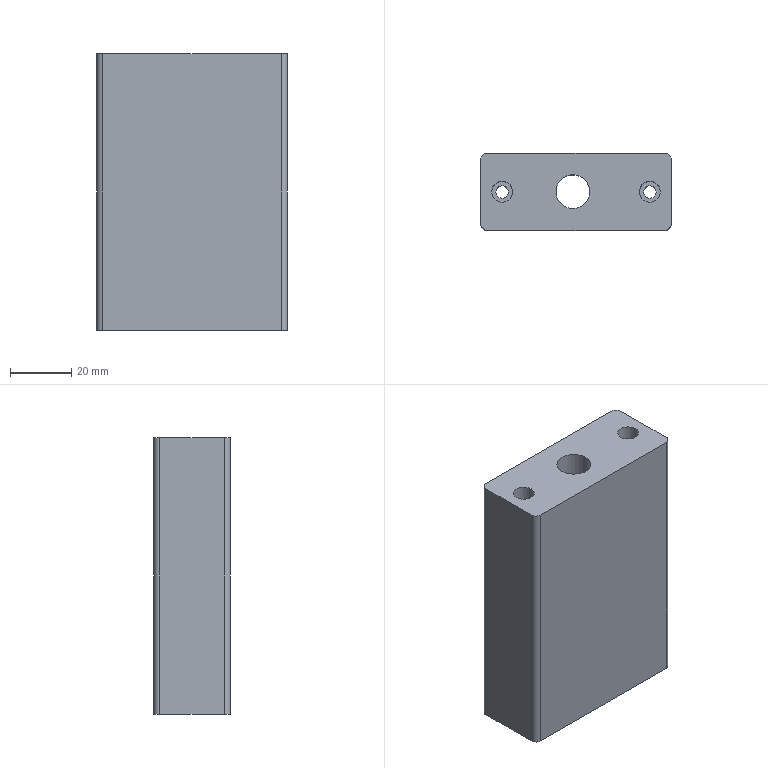Part | STEP file | gslz 2016.10.28-10_id2890_x_t | 1 solid | 19 faces | box 62 x 25 x 90 mm | volume 116529 mm3 | cylinder 10 | plane 9 | commonest cylinder face diameters 4 x4 4.1 x2 6.8 x2 11 x1 17 x1
STEP:
#1=CARTESIAN_POINT('',(0.,0.,0.));
#2=DIRECTION('',(0.,0.,1.));
#3=DIRECTION('',(1.,0.,0.));
#4=AXIS2_PLACEMENT_3D('',#1,#2,#3);
#5=CARTESIAN_POINT('',(1002.,-173.5,85.));
#6=VERTEX_POINT('',#5);
#7=CARTESIAN_POINT('',(1060.,-173.5,85.));
#8=VERTEX_POINT('',#7);
#9=CARTESIAN_POINT('',(1140.635,-173.5,85.));
#10=DIRECTION('',(1.,0.,0.));
#11=VECTOR('',#10,1.);
#12=LINE('',#9,#11);
#13=CARTESIAN_POINT('',(1030.,-162.5,85.));
#14=DIRECTION('',(0.,0.,1.));
#15=DIRECTION('',(-1.,0.,0.));
#16=AXIS2_PLACEMENT_3D('',#13,#14,#15);
#17=PLANE('',#16);
#18=CARTESIAN_POINT('',(-110.635,11.));
#19=DIRECTION('',(-1.,0.));
#20=VECTOR('',#19,1.);
#21=LINE('',#18,#20);
#22=(GEOMETRIC_REPRESENTATION_CONTEXT(2)PARAMETRIC_REPRESENTATION_CONTEXT()REPRESENTATION_CONTEXT('',''));
#23=DEFINITIONAL_REPRESENTATION('',(#21),#22);
#24=PCURVE('',#17,#23);
#25=CARTESIAN_POINT('',(1140.635,-173.5,80.));
#26=DIRECTION('',(0.,1.,0.));
#27=DIRECTION('',(0.,0.,-1.));
#28=AXIS2_PLACEMENT_3D('',#25,#26,#27);
#29=PLANE('',#28);
#30=CARTESIAN_POINT('',(-5.,0.));
#31=DIRECTION('',(0.,-1.));
#32=VECTOR('',#31,1.);
#33=LINE('',#30,#32);
#34=(GEOMETRIC_REPRESENTATION_CONTEXT(2)PARAMETRIC_REPRESENTATION_CONTEXT()REPRESENTATION_CONTEXT('',''));
#35=DEFINITIONAL_REPRESENTATION('',(#33),#34);
#36=PCURVE('',#29,#35);
#37=SURFACE_CURVE('',#12,(#24,#36),.PCURVE_S1.);
#38=EDGE_CURVE('',#6,#8,#37,.T.);
#39=ORIENTED_EDGE('',*,*,#38,.T.);
#40=CARTESIAN_POINT('',(1062.,-171.5,85.));
#41=VERTEX_POINT('',#40);
#42=CARTESIAN_POINT('',(1060.,-171.5,85.));
#43=DIRECTION('',(0.,0.,1.));
#44=DIRECTION('',(1.,0.,0.));
#45=AXIS2_PLACEMENT_3D('',#42,#43,#44);
#46=CIRCLE('',#45,2.);
#47=CARTESIAN_POINT('',(-30.,9.));
#48=DIRECTION('',(-1.,0.));
#49=AXIS2_PLACEMENT_2D('',#47,#48);
#50=CIRCLE('',#49,2.);
#51=(GEOMETRIC_REPRESENTATION_CONTEXT(2)PARAMETRIC_REPRESENTATION_CONTEXT()REPRESENTATION_CONTEXT('',''));
#52=DEFINITIONAL_REPRESENTATION('',(#50),#51);
#53=PCURVE('',#17,#52);
#54=CARTESIAN_POINT('',(1060.,-171.5,80.));
#55=DIRECTION('',(0.,0.,1.));
#56=DIRECTION('',(-1.,0.,0.));
#57=AXIS2_PLACEMENT_3D('',#54,#55,#56);
#58=CYLINDRICAL_SURFACE('',#57,2.);
#59=CARTESIAN_POINT('',(-3.142,5.));
#60=DIRECTION('',(1.,0.));
#61=VECTOR('',#60,1.);
#62=LINE('',#59,#61);
#63=(GEOMETRIC_REPRESENTATION_CONTEXT(2)PARAMETRIC_REPRESENTATION_CONTEXT()REPRESENTATION_CONTEXT('',''));
#64=DEFINITIONAL_REPRESENTATION('',(#62),#63);
#65=PCURVE('',#58,#64);
#66=SURFACE_CURVE('',#46,(#53,#65),.PCURVE_S1.);
#67=EDGE_CURVE('',#8,#41,#66,.T.);
#68=ORIENTED_EDGE('',*,*,#67,.T.);
#69=CARTESIAN_POINT('',(1062.,-150.5,85.));
#70=VERTEX_POINT('',#69);
#71=CARTESIAN_POINT('',(1062.,-161.,85.));
#72=DIRECTION('',(0.,1.,0.));
#73=VECTOR('',#72,1.);
#74=LINE('',#71,#73);
#75=CARTESIAN_POINT('',(-32.,-1.5));
#76=DIRECTION('',(0.,-1.));
#77=VECTOR('',#76,1.);
#78=LINE('',#75,#77);
#79=(GEOMETRIC_REPRESENTATION_CONTEXT(2)PARAMETRIC_REPRESENTATION_CONTEXT()REPRESENTATION_CONTEXT('',''));
#80=DEFINITIONAL_REPRESENTATION('',(#78),#79);
#81=PCURVE('',#17,#80);
#82=CARTESIAN_POINT('',(1062.,-161.,46.));
#83=DIRECTION('',(-1.,0.,0.));
#84=DIRECTION('',(0.,0.,-1.));
#85=AXIS2_PLACEMENT_3D('',#82,#83,#84);
#86=PLANE('',#85);
#87=CARTESIAN_POINT('',(-39.,0.));
#88=DIRECTION('',(0.,-1.));
#89=VECTOR('',#88,1.);
#90=LINE('',#87,#89);
#91=(GEOMETRIC_REPRESENTATION_CONTEXT(2)PARAMETRIC_REPRESENTATION_CONTEXT()REPRESENTATION_CONTEXT('',''));
#92=DEFINITIONAL_REPRESENTATION('',(#90),#91);
#93=PCURVE('',#86,#92);
#94=SURFACE_CURVE('',#74,(#81,#93),.PCURVE_S1.);
#95=EDGE_CURVE('',#41,#70,#94,.T.);
#96=ORIENTED_EDGE('',*,*,#95,.T.);
#97=CARTESIAN_POINT('',(1060.,-148.5,85.));
#98=VERTEX_POINT('',#97);
#99=CARTESIAN_POINT('',(1060.,-150.5,85.));
#100=DIRECTION('',(0.,0.,1.));
#101=DIRECTION('',(1.,0.,0.));
#102=AXIS2_PLACEMENT_3D('',#99,#100,#101);
#103=CIRCLE('',#102,2.);
#104=CARTESIAN_POINT('',(-30.,-12.));
#105=DIRECTION('',(-1.,0.));
#106=AXIS2_PLACEMENT_2D('',#104,#105);
#107=CIRCLE('',#106,2.);
#108=(GEOMETRIC_REPRESENTATION_CONTEXT(2)PARAMETRIC_REPRESENTATION_CONTEXT()REPRESENTATION_CONTEXT('',''));
#109=DEFINITIONAL_REPRESENTATION('',(#107),#108);
#110=PCURVE('',#17,#109);
#111=CARTESIAN_POINT('',(1060.,-150.5,46.));
#112=DIRECTION('',(0.,0.,1.));
#113=DIRECTION('',(-1.,0.,0.));
#114=AXIS2_PLACEMENT_3D('',#111,#112,#113);
#115=CYLINDRICAL_SURFACE('',#114,2.);
#116=CARTESIAN_POINT('',(3.142,39.));
#117=DIRECTION('',(1.,0.));
#118=VECTOR('',#117,1.);
#119=LINE('',#116,#118);
#120=(GEOMETRIC_REPRESENTATION_CONTEXT(2)PARAMETRIC_REPRESENTATION_CONTEXT()REPRESENTATION_CONTEXT('',''));
#121=DEFINITIONAL_REPRESENTATION('',(#119),#120);
#122=PCURVE('',#115,#121);
#123=SURFACE_CURVE('',#103,(#110,#122),.PCURVE_S1.);
#124=EDGE_CURVE('',#70,#98,#123,.T.);
#125=ORIENTED_EDGE('',*,*,#124,.T.);
#126=CARTESIAN_POINT('',(1002.,-148.5,85.));
#127=VERTEX_POINT('',#126);
#128=CARTESIAN_POINT('',(405.,-148.5,85.));
#129=DIRECTION('',(-1.,0.,0.));
#130=VECTOR('',#129,1.);
#131=LINE('',#128,#130);
#132=CARTESIAN_POINT('',(625.,-14.));
#133=DIRECTION('',(1.,0.));
#134=VECTOR('',#133,1.);
#135=LINE('',#132,#134);
#136=(GEOMETRIC_REPRESENTATION_CONTEXT(2)PARAMETRIC_REPRESENTATION_CONTEXT()REPRESENTATION_CONTEXT('',''));
#137=DEFINITIONAL_REPRESENTATION('',(#135),#136);
#138=PCURVE('',#17,#137);
#139=CARTESIAN_POINT('',(405.,-148.5,80.));
#140=DIRECTION('',(0.,-1.,0.));
#141=DIRECTION('',(0.,0.,1.));
#142=AXIS2_PLACEMENT_3D('',#139,#140,#141);
#143=PLANE('',#142);
#144=CARTESIAN_POINT('',(5.,0.));
#145=DIRECTION('',(0.,1.));
#146=VECTOR('',#145,1.);
#147=LINE('',#144,#146);
#148=(GEOMETRIC_REPRESENTATION_CONTEXT(2)PARAMETRIC_REPRESENTATION_CONTEXT()REPRESENTATION_CONTEXT('',''));
#149=DEFINITIONAL_REPRESENTATION('',(#147),#148);
#150=PCURVE('',#143,#149);
#151=SURFACE_CURVE('',#131,(#138,#150),.PCURVE_S1.);
#152=EDGE_CURVE('',#98,#127,#151,.T.);
#153=ORIENTED_EDGE('',*,*,#152,.T.);
#154=CARTESIAN_POINT('',(1000.,-150.5,85.));
#155=VERTEX_POINT('',#154);
#156=CARTESIAN_POINT('',(1002.,-150.5,85.));
#157=DIRECTION('',(0.,0.,1.));
#158=DIRECTION('',(1.,0.,0.));
#159=AXIS2_PLACEMENT_3D('',#156,#157,#158);
#160=CIRCLE('',#159,2.);
#161=CARTESIAN_POINT('',(28.,-12.));
#162=DIRECTION('',(-1.,0.));
#163=AXIS2_PLACEMENT_2D('',#161,#162);
#164=CIRCLE('',#163,2.);
#165=(GEOMETRIC_REPRESENTATION_CONTEXT(2)PARAMETRIC_REPRESENTATION_CONTEXT()REPRESENTATION_CONTEXT('',''));
#166=DEFINITIONAL_REPRESENTATION('',(#164),#165);
#167=PCURVE('',#17,#166);
#168=CARTESIAN_POINT('',(1002.,-150.5,80.));
#169=DIRECTION('',(0.,0.,1.));
#170=DIRECTION('',(-1.,0.,0.));
#171=AXIS2_PLACEMENT_3D('',#168,#169,#170);
#172=CYLINDRICAL_SURFACE('',#171,2.);
#173=CARTESIAN_POINT('',(3.142,5.));
#174=DIRECTION('',(1.,0.));
#175=VECTOR('',#174,1.);
#176=LINE('',#173,#175);
#177=(GEOMETRIC_REPRESENTATION_CONTEXT(2)PARAMETRIC_REPRESENTATION_CONTEXT()REPRESENTATION_CONTEXT('',''));
#178=DEFINITIONAL_REPRESENTATION('',(#176),#177);
#179=PCURVE('',#172,#178);
#180=SURFACE_CURVE('',#160,(#167,#179),.PCURVE_S1.);
#181=EDGE_CURVE('',#127,#155,#180,.T.);
#182=ORIENTED_EDGE('',*,*,#181,.T.);
#183=CARTESIAN_POINT('',(1000.,-171.5,85.));
#184=VERTEX_POINT('',#183);
#185=CARTESIAN_POINT('',(1000.,-154.5,85.));
#186=DIRECTION('',(0.,1.,0.));
#187=VECTOR('',#186,1.);
#188=LINE('',#185,#187);
#189=CARTESIAN_POINT('',(30.,-8.));
#190=DIRECTION('',(0.,-1.));
#191=VECTOR('',#190,1.);
#192=LINE('',#189,#191);
#193=(GEOMETRIC_REPRESENTATION_CONTEXT(2)PARAMETRIC_REPRESENTATION_CONTEXT()REPRESENTATION_CONTEXT('',''));
#194=DEFINITIONAL_REPRESENTATION('',(#192),#193);
#195=PCURVE('',#17,#194);
#196=CARTESIAN_POINT('',(1000.,-154.5,80.));
#197=DIRECTION('',(-1.,0.,0.));
#198=DIRECTION('',(0.,0.,-1.));
#199=AXIS2_PLACEMENT_3D('',#196,#197,#198);
#200=PLANE('',#199);
#201=CARTESIAN_POINT('',(-5.,0.));
#202=DIRECTION('',(0.,-1.));
#203=VECTOR('',#202,1.);
#204=LINE('',#201,#203);
#205=(GEOMETRIC_REPRESENTATION_CONTEXT(2)PARAMETRIC_REPRESENTATION_CONTEXT()REPRESENTATION_CONTEXT('',''));
#206=DEFINITIONAL_REPRESENTATION('',(#204),#205);
#207=PCURVE('',#200,#206);
#208=SURFACE_CURVE('',#188,(#195,#207),.PCURVE_S1.);
#209=EDGE_CURVE('',#184,#155,#208,.T.);
#210=ORIENTED_EDGE('',*,*,#209,.F.);
#211=CARTESIAN_POINT('',(1002.,-171.5,85.));
#212=DIRECTION('',(0.,0.,1.));
#213=DIRECTION('',(1.,0.,0.));
#214=AXIS2_PLACEMENT_3D('',#211,#212,#213);
#215=CIRCLE('',#214,2.);
#216=CARTESIAN_POINT('',(28.,9.));
#217=DIRECTION('',(-1.,0.));
#218=AXIS2_PLACEMENT_2D('',#216,#217);
#219=CIRCLE('',#218,2.);
#220=(GEOMETRIC_REPRESENTATION_CONTEXT(2)PARAMETRIC_REPRESENTATION_CONTEXT()REPRESENTATION_CONTEXT('',''));
#221=DEFINITIONAL_REPRESENTATION('',(#219),#220);
#222=PCURVE('',#17,#221);
#223=CARTESIAN_POINT('',(1002.,-171.5,80.));
#224=DIRECTION('',(0.,0.,1.));
#225=DIRECTION('',(-1.,0.,0.));
#226=AXIS2_PLACEMENT_3D('',#223,#224,#225);
#227=CYLINDRICAL_SURFACE('',#226,2.);
#228=CARTESIAN_POINT('',(-3.142,5.));
#229=DIRECTION('',(1.,0.));
#230=VECTOR('',#229,1.);
#231=LINE('',#228,#230);
#232=(GEOMETRIC_REPRESENTATION_CONTEXT(2)PARAMETRIC_REPRESENTATION_CONTEXT()REPRESENTATION_CONTEXT('',''));
#233=DEFINITIONAL_REPRESENTATION('',(#231),#232);
#234=PCURVE('',#227,#233);
#235=SURFACE_CURVE('',#215,(#222,#234),.PCURVE_S1.);
#236=EDGE_CURVE('',#184,#6,#235,.T.);
#237=ORIENTED_EDGE('',*,*,#236,.T.);
#238=EDGE_LOOP('',(#39,#68,#96,#125,#153,#182,#210,#237));
#239=FACE_BOUND('',#238,.T.);
#240=CARTESIAN_POINT('',(1035.5,-161.,85.));
#241=VERTEX_POINT('',#240);
#242=CARTESIAN_POINT('',(1030.,-161.,85.));
#243=DIRECTION('',(0.,0.,1.));
#244=DIRECTION('',(1.,0.,0.));
#245=AXIS2_PLACEMENT_3D('',#242,#243,#244);
#246=CIRCLE('',#245,5.5);
#247=CARTESIAN_POINT('',(0.,-1.5));
#248=DIRECTION('',(-1.,0.));
#249=AXIS2_PLACEMENT_2D('',#247,#248);
#250=CIRCLE('',#249,5.5);
#251=(GEOMETRIC_REPRESENTATION_CONTEXT(2)PARAMETRIC_REPRESENTATION_CONTEXT()REPRESENTATION_CONTEXT('',''));
#252=DEFINITIONAL_REPRESENTATION('',(#250),#251);
#253=PCURVE('',#17,#252);
#254=CARTESIAN_POINT('',(1030.,-161.,-13.));
#255=DIRECTION('',(0.,0.,1.));
#256=DIRECTION('',(1.,0.,0.));
#257=AXIS2_PLACEMENT_3D('',#254,#255,#256);
#258=CYLINDRICAL_SURFACE('',#257,5.5);
#259=CARTESIAN_POINT('',(0.,98.));
#260=DIRECTION('',(1.,0.));
#261=VECTOR('',#260,1.);
#262=LINE('',#259,#261);
#263=(GEOMETRIC_REPRESENTATION_CONTEXT(2)PARAMETRIC_REPRESENTATION_CONTEXT()REPRESENTATION_CONTEXT('',''));
#264=DEFINITIONAL_REPRESENTATION('',(#262),#263);
#265=PCURVE('',#258,#264);
#266=SURFACE_CURVE('',#246,(#253,#265),.PCURVE_S1.);
#267=EDGE_CURVE('',#241,#241,#266,.T.);
#268=ORIENTED_EDGE('',*,*,#267,.F.);
#269=EDGE_LOOP('',(#268));
#270=FACE_BOUND('',#269,.T.);
#271=CARTESIAN_POINT('',(1010.4,-161.,85.));
#272=VERTEX_POINT('',#271);
#273=CARTESIAN_POINT('',(1007.,-161.,85.));
#274=DIRECTION('',(0.,0.,1.));
#275=DIRECTION('',(1.,0.,0.));
#276=AXIS2_PLACEMENT_3D('',#273,#274,#275);
#277=CIRCLE('',#276,3.4);
#278=CARTESIAN_POINT('',(23.,-1.5));
#279=DIRECTION('',(-1.,0.));
#280=AXIS2_PLACEMENT_2D('',#278,#279);
#281=CIRCLE('',#280,3.4);
#282=(GEOMETRIC_REPRESENTATION_CONTEXT(2)PARAMETRIC_REPRESENTATION_CONTEXT()REPRESENTATION_CONTEXT('',''));
#283=DEFINITIONAL_REPRESENTATION('',(#281),#282);
#284=PCURVE('',#17,#283);
#285=CARTESIAN_POINT('',(1007.,-161.,36.));
#286=DIRECTION('',(0.,0.,1.));
#287=DIRECTION('',(1.,0.,0.));
#288=AXIS2_PLACEMENT_3D('',#285,#286,#287);
#289=CYLINDRICAL_SURFACE('',#288,3.4);
#290=CARTESIAN_POINT('',(0.,49.));
#291=DIRECTION('',(1.,0.));
#292=VECTOR('',#291,1.);
#293=LINE('',#290,#292);
#294=(GEOMETRIC_REPRESENTATION_CONTEXT(2)PARAMETRIC_REPRESENTATION_CONTEXT()REPRESENTATION_CONTEXT('',''));
#295=DEFINITIONAL_REPRESENTATION('',(#293),#294);
#296=PCURVE('',#289,#295);
#297=SURFACE_CURVE('',#277,(#284,#296),.PCURVE_S1.);
#298=EDGE_CURVE('',#272,#272,#297,.T.);
#299=ORIENTED_EDGE('',*,*,#298,.F.);
#300=EDGE_LOOP('',(#299));
#301=FACE_BOUND('',#300,.T.);
#302=CARTESIAN_POINT('',(1058.4,-161.,85.));
#303=VERTEX_POINT('',#302);
#304=CARTESIAN_POINT('',(1055.,-161.,85.));
#305=DIRECTION('',(0.,0.,-1.));
#306=DIRECTION('',(1.,0.,0.));
#307=AXIS2_PLACEMENT_3D('',#304,#305,#306);
#308=CIRCLE('',#307,3.4);
#309=CARTESIAN_POINT('',(-28.4,-1.5));
#310=CARTESIAN_POINT('',(-28.4,4.389));
#311=CARTESIAN_POINT('',(-23.3,1.444));
#312=CARTESIAN_POINT('',(-18.2,-1.5));
#313=CARTESIAN_POINT('',(-23.3,-4.444));
#314=CARTESIAN_POINT('',(-28.4,-7.389));
#315=CARTESIAN_POINT('',(-28.4,-1.5));
#316=(BOUNDED_CURVE()B_SPLINE_CURVE(2,(#309,#310,#311,#312,#313,#314,#315),.UNSPECIFIED.,.T.,.F.)B_SPLINE_CURVE_WITH_KNOTS((1,2,2,2,2,1),(-2.094,0.,2.094,4.189,6.283,8.378),.UNSPECIFIED.)CURVE()GEOMETRIC_REPRESENTATION_ITEM()RATIONAL_B_SPLINE_CURVE((1.,0.5,1.,0.5,1.,0.5,1.))REPRESENTATION_ITEM(''));
#317=(GEOMETRIC_REPRESENTATION_CONTEXT(2)PARAMETRIC_REPRESENTATION_CONTEXT()REPRESENTATION_CONTEXT('',''));
#318=DEFINITIONAL_REPRESENTATION('',(#316),#317);
#319=PCURVE('',#17,#318);
#320=CARTESIAN_POINT('',(1055.,-161.,36.));
#321=DIRECTION('',(0.,0.,1.));
#322=DIRECTION('',(-1.,0.,0.));
#323=AXIS2_PLACEMENT_3D('',#320,#321,#322);
#324=CYLINDRICAL_SURFACE('',#323,3.4);
#325=CARTESIAN_POINT('',(9.425,49.));
#326=DIRECTION('',(-1.,0.));
#327=VECTOR('',#326,1.);
#328=LINE('',#325,#327);
#329=(GEOMETRIC_REPRESENTATION_CONTEXT(2)PARAMETRIC_REPRESENTATION_CONTEXT()REPRESENTATION_CONTEXT('',''));
#330=DEFINITIONAL_REPRESENTATION('',(#328),#329);
#331=PCURVE('',#324,#330);
#332=SURFACE_CURVE('',#308,(#319,#331),.PCURVE_S1.);
#333=EDGE_CURVE('',#303,#303,#332,.T.);
#334=ORIENTED_EDGE('',*,*,#333,.T.);
#335=EDGE_LOOP('',(#334));
#336=FACE_BOUND('',#335,.T.);
#337=ADVANCED_FACE('',(#239,#270,#301,#336),#17,.T.);
#338=CARTESIAN_POINT('',(1052.95,-161.,-5.));
#339=VERTEX_POINT('',#338);
#340=CARTESIAN_POINT('',(1055.,-161.,-5.));
#341=DIRECTION('',(0.,0.,1.));
#342=DIRECTION('',(-1.,0.,0.));
#343=AXIS2_PLACEMENT_3D('',#340,#341,#342);
#344=CIRCLE('',#343,2.05);
#345=CARTESIAN_POINT('',(409.5,-254.354,-5.));
#346=DIRECTION('',(0.,0.,-1.));
#347=DIRECTION('',(1.,0.,0.));
#348=AXIS2_PLACEMENT_3D('',#345,#346,#347);
#349=PLANE('',#348);
#350=CARTESIAN_POINT('',(643.45,-93.354));
#351=CARTESIAN_POINT('',(643.45,-89.804));
#352=CARTESIAN_POINT('',(646.525,-91.579));
#353=CARTESIAN_POINT('',(649.6,-93.354));
#354=CARTESIAN_POINT('',(646.525,-95.13));
#355=CARTESIAN_POINT('',(643.45,-96.905));
#356=CARTESIAN_POINT('',(643.45,-93.354));
#357=(BOUNDED_CURVE()B_SPLINE_CURVE(2,(#350,#351,#352,#353,#354,#355,#356),.UNSPECIFIED.,.T.,.F.)B_SPLINE_CURVE_WITH_KNOTS((1,2,2,2,2,1),(-2.094,0.,2.094,4.189,6.283,8.378),.UNSPECIFIED.)CURVE()GEOMETRIC_REPRESENTATION_ITEM()RATIONAL_B_SPLINE_CURVE((1.,0.5,1.,0.5,1.,0.5,1.))REPRESENTATION_ITEM(''));
#358=(GEOMETRIC_REPRESENTATION_CONTEXT(2)PARAMETRIC_REPRESENTATION_CONTEXT()REPRESENTATION_CONTEXT('',''));
#359=DEFINITIONAL_REPRESENTATION('',(#357),#358);
#360=PCURVE('',#349,#359);
#361=CARTESIAN_POINT('',(1055.,-161.,41.));
#362=DIRECTION('',(0.,0.,-1.));
#363=DIRECTION('',(1.,0.,0.));
#364=AXIS2_PLACEMENT_3D('',#361,#362,#363);
#365=CYLINDRICAL_SURFACE('',#364,2.05);
#366=CARTESIAN_POINT('',(9.425,46.));
#367=DIRECTION('',(-1.,0.));
#368=VECTOR('',#367,1.);
#369=LINE('',#366,#368);
#370=(GEOMETRIC_REPRESENTATION_CONTEXT(2)PARAMETRIC_REPRESENTATION_CONTEXT()REPRESENTATION_CONTEXT('',''));
#371=DEFINITIONAL_REPRESENTATION('',(#369),#370);
#372=PCURVE('',#365,#371);
#373=SURFACE_CURVE('',#344,(#360,#372),.PCURVE_S1.);
#374=EDGE_CURVE('',#339,#339,#373,.T.);
#375=ORIENTED_EDGE('',*,*,#374,.T.);
#376=EDGE_LOOP('',(#375));
#377=FACE_BOUND('',#376,.T.);
#378=CARTESIAN_POINT('',(1004.95,-161.,-5.));
#379=VERTEX_POINT('',#378);
#380=CARTESIAN_POINT('',(1007.,-161.,-5.));
#381=DIRECTION('',(0.,0.,1.));
#382=DIRECTION('',(-1.,0.,0.));
#383=AXIS2_PLACEMENT_3D('',#380,#381,#382);
#384=CIRCLE('',#383,2.05);
#385=CARTESIAN_POINT('',(595.45,-93.354));
#386=CARTESIAN_POINT('',(595.45,-89.804));
#387=CARTESIAN_POINT('',(598.525,-91.579));
#388=CARTESIAN_POINT('',(601.6,-93.354));
#389=CARTESIAN_POINT('',(598.525,-95.13));
#390=CARTESIAN_POINT('',(595.45,-96.905));
#391=CARTESIAN_POINT('',(595.45,-93.354));
#392=(BOUNDED_CURVE()B_SPLINE_CURVE(2,(#385,#386,#387,#388,#389,#390,#391),.UNSPECIFIED.,.T.,.F.)B_SPLINE_CURVE_WITH_KNOTS((1,2,2,2,2,1),(-2.094,0.,2.094,4.189,6.283,8.378),.UNSPECIFIED.)CURVE()GEOMETRIC_REPRESENTATION_ITEM()RATIONAL_B_SPLINE_CURVE((1.,0.5,1.,0.5,1.,0.5,1.))REPRESENTATION_ITEM(''));
#393=(GEOMETRIC_REPRESENTATION_CONTEXT(2)PARAMETRIC_REPRESENTATION_CONTEXT()REPRESENTATION_CONTEXT('',''));
#394=DEFINITIONAL_REPRESENTATION('',(#392),#393);
#395=PCURVE('',#349,#394);
#396=CARTESIAN_POINT('',(1007.,-161.,41.));
#397=DIRECTION('',(0.,0.,-1.));
#398=DIRECTION('',(-1.,0.,0.));
#399=AXIS2_PLACEMENT_3D('',#396,#397,#398);
#400=CYLINDRICAL_SURFACE('',#399,2.05);
#401=CARTESIAN_POINT('',(6.283,46.));
#402=DIRECTION('',(-1.,0.));
#403=VECTOR('',#402,1.);
#404=LINE('',#401,#403);
#405=(GEOMETRIC_REPRESENTATION_CONTEXT(2)PARAMETRIC_REPRESENTATION_CONTEXT()REPRESENTATION_CONTEXT('',''));
#406=DEFINITIONAL_REPRESENTATION('',(#404),#405);
#407=PCURVE('',#400,#406);
#408=SURFACE_CURVE('',#384,(#395,#407),.PCURVE_S1.);
#409=EDGE_CURVE('',#379,#379,#408,.T.);
#410=ORIENTED_EDGE('',*,*,#409,.T.);
#411=EDGE_LOOP('',(#410));
#412=FACE_BOUND('',#411,.T.);
#413=CARTESIAN_POINT('',(1062.,-150.5,-5.));
#414=VERTEX_POINT('',#413);
#415=CARTESIAN_POINT('',(1062.,-171.5,-5.));
#416=VERTEX_POINT('',#415);
#417=CARTESIAN_POINT('',(1062.,-161.,-5.));
#418=DIRECTION('',(0.,-1.,0.));
#419=VECTOR('',#418,1.);
#420=LINE('',#417,#419);
#421=CARTESIAN_POINT('',(652.5,-93.354));
#422=DIRECTION('',(0.,1.));
#423=VECTOR('',#422,1.);
#424=LINE('',#421,#423);
#425=(GEOMETRIC_REPRESENTATION_CONTEXT(2)PARAMETRIC_REPRESENTATION_CONTEXT()REPRESENTATION_CONTEXT('',''));
#426=DEFINITIONAL_REPRESENTATION('',(#424),#425);
#427=PCURVE('',#349,#426);
#428=CARTESIAN_POINT('',(51.,0.));
#429=DIRECTION('',(0.,1.));
#430=VECTOR('',#429,1.);
#431=LINE('',#428,#430);
#432=(GEOMETRIC_REPRESENTATION_CONTEXT(2)PARAMETRIC_REPRESENTATION_CONTEXT()REPRESENTATION_CONTEXT('',''));
#433=DEFINITIONAL_REPRESENTATION('',(#431),#432);
#434=PCURVE('',#86,#433);
#435=SURFACE_CURVE('',#420,(#427,#434),.PCURVE_S1.);
#436=EDGE_CURVE('',#414,#416,#435,.T.);
#437=ORIENTED_EDGE('',*,*,#436,.T.);
#438=CARTESIAN_POINT('',(1060.,-173.5,-5.));
#439=VERTEX_POINT('',#438);
#440=CARTESIAN_POINT('',(1060.,-171.5,-5.));
#441=DIRECTION('',(0.,0.,-1.));
#442=DIRECTION('',(-1.,0.,0.));
#443=AXIS2_PLACEMENT_3D('',#440,#441,#442);
#444=CIRCLE('',#443,2.);
#445=CARTESIAN_POINT('',(650.5,-82.854));
#446=DIRECTION('',(-1.,0.));
#447=AXIS2_PLACEMENT_2D('',#445,#446);
#448=CIRCLE('',#447,2.);
#449=(GEOMETRIC_REPRESENTATION_CONTEXT(2)PARAMETRIC_REPRESENTATION_CONTEXT()REPRESENTATION_CONTEXT('',''));
#450=DEFINITIONAL_REPRESENTATION('',(#448),#449);
#451=PCURVE('',#349,#450);
#452=CARTESIAN_POINT('',(6.283,-85.));
#453=DIRECTION('',(-1.,0.));
#454=VECTOR('',#453,1.);
#455=LINE('',#452,#454);
#456=(GEOMETRIC_REPRESENTATION_CONTEXT(2)PARAMETRIC_REPRESENTATION_CONTEXT()REPRESENTATION_CONTEXT('',''));
#457=DEFINITIONAL_REPRESENTATION('',(#455),#456);
#458=PCURVE('',#58,#457);
#459=SURFACE_CURVE('',#444,(#451,#458),.PCURVE_S1.);
#460=EDGE_CURVE('',#416,#439,#459,.T.);
#461=ORIENTED_EDGE('',*,*,#460,.T.);
#462=CARTESIAN_POINT('',(1002.,-173.5,-5.));
#463=VERTEX_POINT('',#462);
#464=CARTESIAN_POINT('',(409.5,-173.5,-5.));
#465=DIRECTION('',(1.,0.,0.));
#466=VECTOR('',#465,1.);
#467=LINE('',#464,#466);
#468=CARTESIAN_POINT('',(0.,-80.854));
#469=DIRECTION('',(1.,0.));
#470=VECTOR('',#469,1.);
#471=LINE('',#468,#470);
#472=(GEOMETRIC_REPRESENTATION_CONTEXT(2)PARAMETRIC_REPRESENTATION_CONTEXT()REPRESENTATION_CONTEXT('',''));
#473=DEFINITIONAL_REPRESENTATION('',(#471),#472);
#474=PCURVE('',#349,#473);
#475=CARTESIAN_POINT('',(85.,731.135));
#476=DIRECTION('',(0.,-1.));
#477=VECTOR('',#476,1.);
#478=LINE('',#475,#477);
#479=(GEOMETRIC_REPRESENTATION_CONTEXT(2)PARAMETRIC_REPRESENTATION_CONTEXT()REPRESENTATION_CONTEXT('',''));
#480=DEFINITIONAL_REPRESENTATION('',(#478),#479);
#481=PCURVE('',#29,#480);
#482=SURFACE_CURVE('',#467,(#474,#481),.PCURVE_S1.);
#483=EDGE_CURVE('',#463,#439,#482,.T.);
#484=ORIENTED_EDGE('',*,*,#483,.F.);
#485=CARTESIAN_POINT('',(1000.,-171.5,-5.));
#486=VERTEX_POINT('',#485);
#487=CARTESIAN_POINT('',(1002.,-171.5,-5.));
#488=DIRECTION('',(0.,0.,-1.));
#489=DIRECTION('',(-1.,0.,0.));
#490=AXIS2_PLACEMENT_3D('',#487,#488,#489);
#491=CIRCLE('',#490,2.);
#492=CARTESIAN_POINT('',(592.5,-82.854));
#493=DIRECTION('',(-1.,0.));
#494=AXIS2_PLACEMENT_2D('',#492,#493);
#495=CIRCLE('',#494,2.);
#496=(GEOMETRIC_REPRESENTATION_CONTEXT(2)PARAMETRIC_REPRESENTATION_CONTEXT()REPRESENTATION_CONTEXT('',''));
#497=DEFINITIONAL_REPRESENTATION('',(#495),#496);
#498=PCURVE('',#349,#497);
#499=CARTESIAN_POINT('',(6.283,-85.));
#500=DIRECTION('',(-1.,0.));
#501=VECTOR('',#500,1.);
#502=LINE('',#499,#501);
#503=(GEOMETRIC_REPRESENTATION_CONTEXT(2)PARAMETRIC_REPRESENTATION_CONTEXT()REPRESENTATION_CONTEXT('',''));
#504=DEFINITIONAL_REPRESENTATION('',(#502),#503);
#505=PCURVE('',#227,#504);
#506=SURFACE_CURVE('',#491,(#498,#505),.PCURVE_S1.);
#507=EDGE_CURVE('',#463,#486,#506,.T.);
#508=ORIENTED_EDGE('',*,*,#507,.T.);
#509=CARTESIAN_POINT('',(1000.,-150.5,-5.));
#510=VERTEX_POINT('',#509);
#511=CARTESIAN_POINT('',(1000.,-254.354,-5.));
#512=DIRECTION('',(0.,1.,0.));
#513=VECTOR('',#512,1.);
#514=LINE('',#511,#513);
#515=CARTESIAN_POINT('',(590.5,0.));
#516=DIRECTION('',(0.,-1.));
#517=VECTOR('',#516,1.);
#518=LINE('',#515,#517);
#519=(GEOMETRIC_REPRESENTATION_CONTEXT(2)PARAMETRIC_REPRESENTATION_CONTEXT()REPRESENTATION_CONTEXT('',''));
#520=DEFINITIONAL_REPRESENTATION('',(#518),#519);
#521=PCURVE('',#349,#520);
#522=CARTESIAN_POINT('',(85.,99.854));
#523=DIRECTION('',(0.,-1.));
#524=VECTOR('',#523,1.);
#525=LINE('',#522,#524);
#526=(GEOMETRIC_REPRESENTATION_CONTEXT(2)PARAMETRIC_REPRESENTATION_CONTEXT()REPRESENTATION_CONTEXT('',''));
#527=DEFINITIONAL_REPRESENTATION('',(#525),#526);
#528=PCURVE('',#200,#527);
#529=SURFACE_CURVE('',#514,(#521,#528),.PCURVE_S1.);
#530=EDGE_CURVE('',#486,#510,#529,.T.);
#531=ORIENTED_EDGE('',*,*,#530,.T.);
#532=CARTESIAN_POINT('',(1002.,-148.5,-5.));
#533=VERTEX_POINT('',#532);
#534=CARTESIAN_POINT('',(1002.,-150.5,-5.));
#535=DIRECTION('',(0.,0.,-1.));
#536=DIRECTION('',(-1.,0.,0.));
#537=AXIS2_PLACEMENT_3D('',#534,#535,#536);
#538=CIRCLE('',#537,2.);
#539=CARTESIAN_POINT('',(592.5,-103.854));
#540=DIRECTION('',(-1.,0.));
#541=AXIS2_PLACEMENT_2D('',#539,#540);
#542=CIRCLE('',#541,2.);
#543=(GEOMETRIC_REPRESENTATION_CONTEXT(2)PARAMETRIC_REPRESENTATION_CONTEXT()REPRESENTATION_CONTEXT('',''));
#544=DEFINITIONAL_REPRESENTATION('',(#542),#543);
#545=PCURVE('',#349,#544);
#546=CARTESIAN_POINT('',(6.283,-85.));
#547=DIRECTION('',(-1.,0.));
#548=VECTOR('',#547,1.);
#549=LINE('',#546,#548);
#550=(GEOMETRIC_REPRESENTATION_CONTEXT(2)PARAMETRIC_REPRESENTATION_CONTEXT()REPRESENTATION_CONTEXT('',''));
#551=DEFINITIONAL_REPRESENTATION('',(#549),#550);
#552=PCURVE('',#172,#551);
#553=SURFACE_CURVE('',#538,(#545,#552),.PCURVE_S1.);
#554=EDGE_CURVE('',#510,#533,#553,.T.);
#555=ORIENTED_EDGE('',*,*,#554,.T.);
#556=CARTESIAN_POINT('',(1060.,-148.5,-5.));
#557=VERTEX_POINT('',#556);
#558=CARTESIAN_POINT('',(409.5,-148.5,-5.));
#559=DIRECTION('',(-1.,0.,0.));
#560=VECTOR('',#559,1.);
#561=LINE('',#558,#560);
#562=CARTESIAN_POINT('',(0.,-105.854));
#563=DIRECTION('',(-1.,0.));
#564=VECTOR('',#563,1.);
#565=LINE('',#562,#564);
#566=(GEOMETRIC_REPRESENTATION_CONTEXT(2)PARAMETRIC_REPRESENTATION_CONTEXT()REPRESENTATION_CONTEXT('',''));
#567=DEFINITIONAL_REPRESENTATION('',(#565),#566);
#568=PCURVE('',#349,#567);
#569=CARTESIAN_POINT('',(-85.,-4.5));
#570=DIRECTION('',(0.,1.));
#571=VECTOR('',#570,1.);
#572=LINE('',#569,#571);
#573=(GEOMETRIC_REPRESENTATION_CONTEXT(2)PARAMETRIC_REPRESENTATION_CONTEXT()REPRESENTATION_CONTEXT('',''));
#574=DEFINITIONAL_REPRESENTATION('',(#572),#573);
#575=PCURVE('',#143,#574);
#576=SURFACE_CURVE('',#561,(#568,#575),.PCURVE_S1.);
#577=EDGE_CURVE('',#557,#533,#576,.T.);
#578=ORIENTED_EDGE('',*,*,#577,.F.);
#579=CARTESIAN_POINT('',(1060.,-150.5,-5.));
#580=DIRECTION('',(0.,0.,-1.));
#581=DIRECTION('',(-1.,0.,0.));
#582=AXIS2_PLACEMENT_3D('',#579,#580,#581);
#583=CIRCLE('',#582,2.);
#584=CARTESIAN_POINT('',(650.5,-103.854));
#585=DIRECTION('',(-1.,0.));
#586=AXIS2_PLACEMENT_2D('',#584,#585);
#587=CIRCLE('',#586,2.);
#588=(GEOMETRIC_REPRESENTATION_CONTEXT(2)PARAMETRIC_REPRESENTATION_CONTEXT()REPRESENTATION_CONTEXT('',''));
#589=DEFINITIONAL_REPRESENTATION('',(#587),#588);
#590=PCURVE('',#349,#589);
#591=CARTESIAN_POINT('',(6.283,-51.));
#592=DIRECTION('',(-1.,0.));
#593=VECTOR('',#592,1.);
#594=LINE('',#591,#593);
#595=(GEOMETRIC_REPRESENTATION_CONTEXT(2)PARAMETRIC_REPRESENTATION_CONTEXT()REPRESENTATION_CONTEXT('',''));
#596=DEFINITIONAL_REPRESENTATION('',(#594),#595);
#597=PCURVE('',#115,#596);
#598=SURFACE_CURVE('',#583,(#590,#597),.PCURVE_S1.);
#599=EDGE_CURVE('',#557,#414,#598,.T.);
#600=ORIENTED_EDGE('',*,*,#599,.T.);
#601=EDGE_LOOP('',(#437,#461,#484,#508,#531,#555,#578,#600));
#602=FACE_BOUND('',#601,.T.);
#603=CARTESIAN_POINT('',(1021.5,-161.,-5.));
#604=VERTEX_POINT('',#603);
#605=CARTESIAN_POINT('',(1038.5,-161.,-5.));
#606=VERTEX_POINT('',#605);
#607=CARTESIAN_POINT('',(1030.,-161.,-5.));
#608=DIRECTION('',(0.,0.,-1.));
#609=DIRECTION('',(-1.,0.,0.));
#610=AXIS2_PLACEMENT_3D('',#607,#608,#609);
#611=CIRCLE('',#610,8.5);
#612=CARTESIAN_POINT('',(620.5,-93.354));
#613=DIRECTION('',(-1.,0.));
#614=AXIS2_PLACEMENT_2D('',#612,#613);
#615=CIRCLE('',#614,8.5);
#616=(GEOMETRIC_REPRESENTATION_CONTEXT(2)PARAMETRIC_REPRESENTATION_CONTEXT()REPRESENTATION_CONTEXT('',''));
#617=DEFINITIONAL_REPRESENTATION('',(#615),#616);
#618=PCURVE('',#349,#617);
#619=CARTESIAN_POINT('',(1030.,-161.,-8.));
#620=DIRECTION('',(0.,0.,1.));
#621=DIRECTION('',(1.,0.,0.));
#622=AXIS2_PLACEMENT_3D('',#619,#620,#621);
#623=CYLINDRICAL_SURFACE('',#622,8.5);
#624=CARTESIAN_POINT('',(3.142,3.));
#625=DIRECTION('',(-1.,0.));
#626=VECTOR('',#625,1.);
#627=LINE('',#624,#626);
#628=(GEOMETRIC_REPRESENTATION_CONTEXT(2)PARAMETRIC_REPRESENTATION_CONTEXT()REPRESENTATION_CONTEXT('',''));
#629=DEFINITIONAL_REPRESENTATION('',(#627),#628);
#630=PCURVE('',#623,#629);
#631=SURFACE_CURVE('',#611,(#618,#630),.PCURVE_S1.);
#632=EDGE_CURVE('',#604,#606,#631,.T.);
#633=ORIENTED_EDGE('',*,*,#632,.F.);
#634=CARTESIAN_POINT('',(1030.,-161.,-5.));
#635=DIRECTION('',(0.,0.,-1.));
#636=DIRECTION('',(-1.,0.,0.));
#637=AXIS2_PLACEMENT_3D('',#634,#635,#636);
#638=CIRCLE('',#637,8.5);
#639=CARTESIAN_POINT('',(620.5,-93.354));
#640=DIRECTION('',(-1.,0.));
#641=AXIS2_PLACEMENT_2D('',#639,#640);
#642=CIRCLE('',#641,8.5);
#643=(GEOMETRIC_REPRESENTATION_CONTEXT(2)PARAMETRIC_REPRESENTATION_CONTEXT()REPRESENTATION_CONTEXT('',''));
#644=DEFINITIONAL_REPRESENTATION('',(#642),#643);
#645=PCURVE('',#349,#644);
#646=CARTESIAN_POINT('',(9.425,3.));
#647=DIRECTION('',(-1.,0.));
#648=VECTOR('',#647,1.);
#649=LINE('',#646,#648);
#650=(GEOMETRIC_REPRESENTATION_CONTEXT(2)PARAMETRIC_REPRESENTATION_CONTEXT()REPRESENTATION_CONTEXT('',''));
#651=DEFINITIONAL_REPRESENTATION('',(#649),#650);
#652=PCURVE('',#623,#651);
#653=SURFACE_CURVE('',#638,(#645,#652),.PCURVE_S1.);
#654=EDGE_CURVE('',#606,#604,#653,.T.);
#655=ORIENTED_EDGE('',*,*,#654,.F.);
#656=EDGE_LOOP('',(#633,#655));
#657=FACE_BOUND('',#656,.T.);
#658=ADVANCED_FACE('',(#377,#412,#602,#657),#349,.T.);
#659=ORIENTED_EDGE('',*,*,#152,.F.);
#660=CARTESIAN_POINT('',(1060.,-148.5,80.));
#661=DIRECTION('',(0.,0.,-1.));
#662=VECTOR('',#661,1.);
#663=LINE('',#660,#662);
#664=CARTESIAN_POINT('',(0.,-655.));
#665=DIRECTION('',(-1.,0.));
#666=VECTOR('',#665,1.);
#667=LINE('',#664,#666);
#668=(GEOMETRIC_REPRESENTATION_CONTEXT(2)PARAMETRIC_REPRESENTATION_CONTEXT()REPRESENTATION_CONTEXT('',''));
#669=DEFINITIONAL_REPRESENTATION('',(#667),#668);
#670=PCURVE('',#143,#669);
#671=CARTESIAN_POINT('',(4.712,34.));
#672=DIRECTION('',(0.,-1.));
#673=VECTOR('',#672,1.);
#674=LINE('',#671,#673);
#675=(GEOMETRIC_REPRESENTATION_CONTEXT(2)PARAMETRIC_REPRESENTATION_CONTEXT()REPRESENTATION_CONTEXT('',''));
#676=DEFINITIONAL_REPRESENTATION('',(#674),#675);
#677=PCURVE('',#115,#676);
#678=SURFACE_CURVE('',#663,(#670,#677),.PCURVE_S1.);
#679=EDGE_CURVE('',#98,#557,#678,.T.);
#680=ORIENTED_EDGE('',*,*,#679,.T.);
#681=ORIENTED_EDGE('',*,*,#577,.T.);
#682=CARTESIAN_POINT('',(1002.,-148.5,100.));
#683=DIRECTION('',(0.,0.,1.));
#684=VECTOR('',#683,1.);
#685=LINE('',#682,#684);
#686=CARTESIAN_POINT('',(20.,-597.));
#687=DIRECTION('',(1.,0.));
#688=VECTOR('',#687,1.);
#689=LINE('',#686,#688);
#690=(GEOMETRIC_REPRESENTATION_CONTEXT(2)PARAMETRIC_REPRESENTATION_CONTEXT()REPRESENTATION_CONTEXT('',''));
#691=DEFINITIONAL_REPRESENTATION('',(#689),#690);
#692=PCURVE('',#143,#691);
#693=CARTESIAN_POINT('',(4.712,20.));
#694=DIRECTION('',(0.,1.));
#695=VECTOR('',#694,1.);
#696=LINE('',#693,#695);
#697=(GEOMETRIC_REPRESENTATION_CONTEXT(2)PARAMETRIC_REPRESENTATION_CONTEXT()REPRESENTATION_CONTEXT('',''));
#698=DEFINITIONAL_REPRESENTATION('',(#696),#697);
#699=PCURVE('',#172,#698);
#700=SURFACE_CURVE('',#685,(#692,#699),.PCURVE_S1.);
#701=EDGE_CURVE('',#533,#127,#700,.T.);
#702=ORIENTED_EDGE('',*,*,#701,.T.);
#703=EDGE_LOOP('',(#659,#680,#681,#702));
#704=FACE_BOUND('',#703,.T.);
#705=ADVANCED_FACE('',(#704),#143,.F.);
#706=ORIENTED_EDGE('',*,*,#209,.T.);
#707=CARTESIAN_POINT('',(1000.,-150.5,-8.));
#708=DIRECTION('',(0.,0.,-1.));
#709=VECTOR('',#708,1.);
#710=LINE('',#707,#709);
#711=CARTESIAN_POINT('',(88.,-4.));
#712=DIRECTION('',(1.,0.));
#713=VECTOR('',#712,1.);
#714=LINE('',#711,#713);
#715=(GEOMETRIC_REPRESENTATION_CONTEXT(2)PARAMETRIC_REPRESENTATION_CONTEXT()REPRESENTATION_CONTEXT('',''));
#716=DEFINITIONAL_REPRESENTATION('',(#714),#715);
#717=PCURVE('',#200,#716);
#718=CARTESIAN_POINT('',(6.283,-88.));
#719=DIRECTION('',(0.,-1.));
#720=VECTOR('',#719,1.);
#721=LINE('',#718,#720);
#722=(GEOMETRIC_REPRESENTATION_CONTEXT(2)PARAMETRIC_REPRESENTATION_CONTEXT()REPRESENTATION_CONTEXT('',''));
#723=DEFINITIONAL_REPRESENTATION('',(#721),#722);
#724=PCURVE('',#172,#723);
#725=SURFACE_CURVE('',#710,(#717,#724),.PCURVE_S1.);
#726=EDGE_CURVE('',#155,#510,#725,.T.);
#727=ORIENTED_EDGE('',*,*,#726,.T.);
#728=ORIENTED_EDGE('',*,*,#530,.F.);
#729=CARTESIAN_POINT('',(1000.,-171.5,100.));
#730=DIRECTION('',(0.,0.,1.));
#731=VECTOR('',#730,1.);
#732=LINE('',#729,#731);
#733=CARTESIAN_POINT('',(-20.,17.));
#734=DIRECTION('',(-1.,0.));
#735=VECTOR('',#734,1.);
#736=LINE('',#733,#735);
#737=(GEOMETRIC_REPRESENTATION_CONTEXT(2)PARAMETRIC_REPRESENTATION_CONTEXT()REPRESENTATION_CONTEXT('',''));
#738=DEFINITIONAL_REPRESENTATION('',(#736),#737);
#739=PCURVE('',#200,#738);
#740=CARTESIAN_POINT('',(0.,20.));
#741=DIRECTION('',(0.,1.));
#742=VECTOR('',#741,1.);
#743=LINE('',#740,#742);
#744=(GEOMETRIC_REPRESENTATION_CONTEXT(2)PARAMETRIC_REPRESENTATION_CONTEXT()REPRESENTATION_CONTEXT('',''));
#745=DEFINITIONAL_REPRESENTATION('',(#743),#744);
#746=PCURVE('',#227,#745);
#747=SURFACE_CURVE('',#732,(#739,#746),.PCURVE_S1.);
#748=EDGE_CURVE('',#486,#184,#747,.T.);
#749=ORIENTED_EDGE('',*,*,#748,.T.);
#750=EDGE_LOOP('',(#706,#727,#728,#749));
#751=FACE_BOUND('',#750,.T.);
#752=ADVANCED_FACE('',(#751),#200,.T.);
#753=ORIENTED_EDGE('',*,*,#483,.T.);
#754=CARTESIAN_POINT('',(1060.,-173.5,80.));
#755=DIRECTION('',(0.,0.,1.));
#756=VECTOR('',#755,1.);
#757=LINE('',#754,#756);
#758=CARTESIAN_POINT('',(0.,80.635));
#759=DIRECTION('',(-1.,0.));
#760=VECTOR('',#759,1.);
#761=LINE('',#758,#760);
#762=(GEOMETRIC_REPRESENTATION_CONTEXT(2)PARAMETRIC_REPRESENTATION_CONTEXT()REPRESENTATION_CONTEXT('',''));
#763=DEFINITIONAL_REPRESENTATION('',(#761),#762);
#764=PCURVE('',#29,#763);
#765=CARTESIAN_POINT('',(1.571,0.));
#766=DIRECTION('',(0.,1.));
#767=VECTOR('',#766,1.);
#768=LINE('',#765,#767);
#769=(GEOMETRIC_REPRESENTATION_CONTEXT(2)PARAMETRIC_REPRESENTATION_CONTEXT()REPRESENTATION_CONTEXT('',''));
#770=DEFINITIONAL_REPRESENTATION('',(#768),#769);
#771=PCURVE('',#58,#770);
#772=SURFACE_CURVE('',#757,(#764,#771),.PCURVE_S1.);
#773=EDGE_CURVE('',#439,#8,#772,.T.);
#774=ORIENTED_EDGE('',*,*,#773,.T.);
#775=ORIENTED_EDGE('',*,*,#38,.F.);
#776=CARTESIAN_POINT('',(1002.,-173.5,-8.));
#777=DIRECTION('',(0.,0.,-1.));
#778=VECTOR('',#777,1.);
#779=LINE('',#776,#778);
#780=CARTESIAN_POINT('',(88.,138.635));
#781=DIRECTION('',(1.,0.));
#782=VECTOR('',#781,1.);
#783=LINE('',#780,#782);
#784=(GEOMETRIC_REPRESENTATION_CONTEXT(2)PARAMETRIC_REPRESENTATION_CONTEXT()REPRESENTATION_CONTEXT('',''));
#785=DEFINITIONAL_REPRESENTATION('',(#783),#784);
#786=PCURVE('',#29,#785);
#787=CARTESIAN_POINT('',(1.571,-88.));
#788=DIRECTION('',(0.,-1.));
#789=VECTOR('',#788,1.);
#790=LINE('',#787,#789);
#791=(GEOMETRIC_REPRESENTATION_CONTEXT(2)PARAMETRIC_REPRESENTATION_CONTEXT()REPRESENTATION_CONTEXT('',''));
#792=DEFINITIONAL_REPRESENTATION('',(#790),#791);
#793=PCURVE('',#227,#792);
#794=SURFACE_CURVE('',#779,(#786,#793),.PCURVE_S1.);
#795=EDGE_CURVE('',#6,#463,#794,.T.);
#796=ORIENTED_EDGE('',*,*,#795,.T.);
#797=EDGE_LOOP('',(#753,#774,#775,#796));
#798=FACE_BOUND('',#797,.T.);
#799=ADVANCED_FACE('',(#798),#29,.F.);
#800=ORIENTED_EDGE('',*,*,#95,.F.);
#801=CARTESIAN_POINT('',(1062.,-171.5,46.));
#802=DIRECTION('',(0.,0.,-1.));
#803=VECTOR('',#802,1.);
#804=LINE('',#801,#803);
#805=CARTESIAN_POINT('',(0.,10.5));
#806=DIRECTION('',(1.,0.));
#807=VECTOR('',#806,1.);
#808=LINE('',#805,#807);
#809=(GEOMETRIC_REPRESENTATION_CONTEXT(2)PARAMETRIC_REPRESENTATION_CONTEXT()REPRESENTATION_CONTEXT('',''));
#810=DEFINITIONAL_REPRESENTATION('',(#808),#809);
#811=PCURVE('',#86,#810);
#812=CARTESIAN_POINT('',(3.142,-34.));
#813=DIRECTION('',(0.,-1.));
#814=VECTOR('',#813,1.);
#815=LINE('',#812,#814);
#816=(GEOMETRIC_REPRESENTATION_CONTEXT(2)PARAMETRIC_REPRESENTATION_CONTEXT()REPRESENTATION_CONTEXT('',''));
#817=DEFINITIONAL_REPRESENTATION('',(#815),#816);
#818=PCURVE('',#58,#817);
#819=SURFACE_CURVE('',#804,(#811,#818),.PCURVE_S1.);
#820=EDGE_CURVE('',#41,#416,#819,.T.);
#821=ORIENTED_EDGE('',*,*,#820,.T.);
#822=ORIENTED_EDGE('',*,*,#436,.F.);
#823=CARTESIAN_POINT('',(1062.,-150.5,46.));
#824=DIRECTION('',(0.,0.,1.));
#825=VECTOR('',#824,1.);
#826=LINE('',#823,#825);
#827=CARTESIAN_POINT('',(0.,-10.5));
#828=DIRECTION('',(-1.,0.));
#829=VECTOR('',#828,1.);
#830=LINE('',#827,#829);
#831=(GEOMETRIC_REPRESENTATION_CONTEXT(2)PARAMETRIC_REPRESENTATION_CONTEXT()REPRESENTATION_CONTEXT('',''));
#832=DEFINITIONAL_REPRESENTATION('',(#830),#831);
#833=PCURVE('',#86,#832);
#834=CARTESIAN_POINT('',(3.142,0.));
#835=DIRECTION('',(0.,1.));
#836=VECTOR('',#835,1.);
#837=LINE('',#834,#836);
#838=(GEOMETRIC_REPRESENTATION_CONTEXT(2)PARAMETRIC_REPRESENTATION_CONTEXT()REPRESENTATION_CONTEXT('',''));
#839=DEFINITIONAL_REPRESENTATION('',(#837),#838);
#840=PCURVE('',#115,#839);
#841=SURFACE_CURVE('',#826,(#833,#840),.PCURVE_S1.);
#842=EDGE_CURVE('',#414,#70,#841,.T.);
#843=ORIENTED_EDGE('',*,*,#842,.T.);
#844=EDGE_LOOP('',(#800,#821,#822,#843));
#845=FACE_BOUND('',#844,.T.);
#846=ADVANCED_FACE('',(#845),#86,.F.);
#847=ORIENTED_EDGE('',*,*,#460,.F.);
#848=ORIENTED_EDGE('',*,*,#820,.F.);
#849=ORIENTED_EDGE('',*,*,#67,.F.);
#850=ORIENTED_EDGE('',*,*,#773,.F.);
#851=EDGE_LOOP('',(#847,#848,#849,#850));
#852=FACE_BOUND('',#851,.T.);
#853=ADVANCED_FACE('',(#852),#58,.T.);
#854=ORIENTED_EDGE('',*,*,#599,.F.);
#855=ORIENTED_EDGE('',*,*,#679,.F.);
#856=ORIENTED_EDGE('',*,*,#124,.F.);
#857=ORIENTED_EDGE('',*,*,#842,.F.);
#858=EDGE_LOOP('',(#854,#855,#856,#857));
#859=FACE_BOUND('',#858,.T.);
#860=ADVANCED_FACE('',(#859),#115,.T.);
#861=ORIENTED_EDGE('',*,*,#181,.F.);
#862=ORIENTED_EDGE('',*,*,#701,.F.);
#863=ORIENTED_EDGE('',*,*,#554,.F.);
#864=ORIENTED_EDGE('',*,*,#726,.F.);
#865=EDGE_LOOP('',(#861,#862,#863,#864));
#866=FACE_BOUND('',#865,.T.);
#867=ADVANCED_FACE('',(#866),#172,.T.);
#868=ORIENTED_EDGE('',*,*,#236,.F.);
#869=ORIENTED_EDGE('',*,*,#748,.F.);
#870=ORIENTED_EDGE('',*,*,#507,.F.);
#871=ORIENTED_EDGE('',*,*,#795,.F.);
#872=EDGE_LOOP('',(#868,#869,#870,#871));
#873=FACE_BOUND('',#872,.T.);
#874=ADVANCED_FACE('',(#873),#227,.T.);
#875=CARTESIAN_POINT('',(1035.5,-161.,65.));
#876=VERTEX_POINT('',#875);
#877=CARTESIAN_POINT('',(1030.,-161.,65.));
#878=DIRECTION('',(0.,0.,-1.));
#879=DIRECTION('',(1.,0.,0.));
#880=AXIS2_PLACEMENT_3D('',#877,#878,#879);
#881=CIRCLE('',#880,5.5);
#882=CARTESIAN_POINT('',(6.283,78.));
#883=DIRECTION('',(-1.,0.));
#884=VECTOR('',#883,1.);
#885=LINE('',#882,#884);
#886=(GEOMETRIC_REPRESENTATION_CONTEXT(2)PARAMETRIC_REPRESENTATION_CONTEXT()REPRESENTATION_CONTEXT('',''));
#887=DEFINITIONAL_REPRESENTATION('',(#885),#886);
#888=PCURVE('',#258,#887);
#889=CARTESIAN_POINT('',(1030.,-162.5,65.));
#890=DIRECTION('',(0.,0.,1.));
#891=DIRECTION('',(-1.,0.,0.));
#892=AXIS2_PLACEMENT_3D('',#889,#890,#891);
#893=PLANE('',#892);
#894=CARTESIAN_POINT('',(-5.5,-1.5));
#895=CARTESIAN_POINT('',(-5.5,8.026));
#896=CARTESIAN_POINT('',(2.75,3.263));
#897=CARTESIAN_POINT('',(11.,-1.5));
#898=CARTESIAN_POINT('',(2.75,-6.263));
#899=CARTESIAN_POINT('',(-5.5,-11.026));
#900=CARTESIAN_POINT('',(-5.5,-1.5));
#901=(BOUNDED_CURVE()B_SPLINE_CURVE(2,(#894,#895,#896,#897,#898,#899,#900),.UNSPECIFIED.,.T.,.F.)B_SPLINE_CURVE_WITH_KNOTS((1,2,2,2,2,1),(-2.094,0.,2.094,4.189,6.283,8.378),.UNSPECIFIED.)CURVE()GEOMETRIC_REPRESENTATION_ITEM()RATIONAL_B_SPLINE_CURVE((1.,0.5,1.,0.5,1.,0.5,1.))REPRESENTATION_ITEM(''));
#902=(GEOMETRIC_REPRESENTATION_CONTEXT(2)PARAMETRIC_REPRESENTATION_CONTEXT()REPRESENTATION_CONTEXT('',''));
#903=DEFINITIONAL_REPRESENTATION('',(#901),#902);
#904=PCURVE('',#893,#903);
#905=SURFACE_CURVE('',#881,(#888,#904),.PCURVE_S1.);
#906=EDGE_CURVE('',#876,#876,#905,.T.);
#907=ORIENTED_EDGE('',*,*,#906,.F.);
#908=CARTESIAN_POINT('',(1035.5,-161.,65.));
#909=CARTESIAN_POINT('',(1035.5,-161.,85.));
#910=B_SPLINE_CURVE_WITH_KNOTS('',1,(#908,#909),.UNSPECIFIED.,.F.,.F.,(2,2),(78.,98.),.PIECEWISE_BEZIER_KNOTS.);
#911=CARTESIAN_POINT('',(6.283,0.));
#912=DIRECTION('',(0.,1.));
#913=VECTOR('',#912,1.);
#914=LINE('',#911,#913);
#915=(GEOMETRIC_REPRESENTATION_CONTEXT(2)PARAMETRIC_REPRESENTATION_CONTEXT()REPRESENTATION_CONTEXT('',''));
#916=DEFINITIONAL_REPRESENTATION('',(#914),#915);
#917=PCURVE('',#258,#916);
#918=CARTESIAN_POINT('',(0.,0.));
#919=DIRECTION('',(0.,1.));
#920=VECTOR('',#919,1.);
#921=LINE('',#918,#920);
#922=(GEOMETRIC_REPRESENTATION_CONTEXT(2)PARAMETRIC_REPRESENTATION_CONTEXT()REPRESENTATION_CONTEXT('',''));
#923=DEFINITIONAL_REPRESENTATION('',(#921),#922);
#924=PCURVE('',#258,#923);
#925=SEAM_CURVE('',#910,(#917,#924),.PCURVE_S1.);
#926=EDGE_CURVE('',#876,#241,#925,.T.);
#927=ORIENTED_EDGE('',*,*,#926,.T.);
#928=ORIENTED_EDGE('',*,*,#267,.F.);
#929=ORIENTED_EDGE('',*,*,#926,.F.);
#930=EDGE_LOOP('',(#907,#927,#928,#929));
#931=FACE_BOUND('',#930,.F.);
#932=ADVANCED_FACE('',(#931),#258,.F.);
#933=ORIENTED_EDGE('',*,*,#906,.F.);
#934=EDGE_LOOP('',(#933));
#935=FACE_BOUND('',#934,.T.);
#936=CARTESIAN_POINT('',(1038.5,-161.,65.));
#937=VERTEX_POINT('',#936);
#938=CARTESIAN_POINT('',(1030.,-161.,65.));
#939=DIRECTION('',(0.,0.,-1.));
#940=DIRECTION('',(1.,0.,0.));
#941=AXIS2_PLACEMENT_3D('',#938,#939,#940);
#942=CIRCLE('',#941,8.5);
#943=CARTESIAN_POINT('',(-8.5,-1.5));
#944=CARTESIAN_POINT('',(-8.5,13.222));
#945=CARTESIAN_POINT('',(4.25,5.861));
#946=CARTESIAN_POINT('',(17.,-1.5));
#947=CARTESIAN_POINT('',(4.25,-8.861));
#948=CARTESIAN_POINT('',(-8.5,-16.222));
#949=CARTESIAN_POINT('',(-8.5,-1.5));
#950=(BOUNDED_CURVE()B_SPLINE_CURVE(2,(#943,#944,#945,#946,#947,#948,#949),.UNSPECIFIED.,.T.,.F.)B_SPLINE_CURVE_WITH_KNOTS((1,2,2,2,2,1),(-2.094,0.,2.094,4.189,6.283,8.378),.UNSPECIFIED.)CURVE()GEOMETRIC_REPRESENTATION_ITEM()RATIONAL_B_SPLINE_CURVE((1.,0.5,1.,0.5,1.,0.5,1.))REPRESENTATION_ITEM(''));
#951=(GEOMETRIC_REPRESENTATION_CONTEXT(2)PARAMETRIC_REPRESENTATION_CONTEXT()REPRESENTATION_CONTEXT('',''));
#952=DEFINITIONAL_REPRESENTATION('',(#950),#951);
#953=PCURVE('',#893,#952);
#954=CARTESIAN_POINT('',(6.283,73.));
#955=DIRECTION('',(-1.,0.));
#956=VECTOR('',#955,1.);
#957=LINE('',#954,#956);
#958=(GEOMETRIC_REPRESENTATION_CONTEXT(2)PARAMETRIC_REPRESENTATION_CONTEXT()REPRESENTATION_CONTEXT('',''));
#959=DEFINITIONAL_REPRESENTATION('',(#957),#958);
#960=PCURVE('',#623,#959);
#961=SURFACE_CURVE('',#942,(#953,#960),.PCURVE_S1.);
#962=EDGE_CURVE('',#937,#937,#961,.T.);
#963=ORIENTED_EDGE('',*,*,#962,.T.);
#964=EDGE_LOOP('',(#963));
#965=FACE_BOUND('',#964,.T.);
#966=ADVANCED_FACE('',(#935,#965),#893,.F.);
#967=ORIENTED_EDGE('',*,*,#962,.T.);
#968=CARTESIAN_POINT('',(1038.5,-161.,-5.));
#969=CARTESIAN_POINT('',(1038.5,-161.,65.));
#970=B_SPLINE_CURVE_WITH_KNOTS('',1,(#968,#969),.UNSPECIFIED.,.F.,.F.,(2,2),(3.,73.),.PIECEWISE_BEZIER_KNOTS.);
#971=CARTESIAN_POINT('',(0.,0.));
#972=DIRECTION('',(0.,1.));
#973=VECTOR('',#972,1.);
#974=LINE('',#971,#973);
#975=(GEOMETRIC_REPRESENTATION_CONTEXT(2)PARAMETRIC_REPRESENTATION_CONTEXT()REPRESENTATION_CONTEXT('',''));
#976=DEFINITIONAL_REPRESENTATION('',(#974),#975);
#977=PCURVE('',#623,#976);
#978=CARTESIAN_POINT('',(6.283,0.));
#979=DIRECTION('',(0.,1.));
#980=VECTOR('',#979,1.);
#981=LINE('',#978,#980);
#982=(GEOMETRIC_REPRESENTATION_CONTEXT(2)PARAMETRIC_REPRESENTATION_CONTEXT()REPRESENTATION_CONTEXT('',''));
#983=DEFINITIONAL_REPRESENTATION('',(#981),#982);
#984=PCURVE('',#623,#983);
#985=SEAM_CURVE('',#970,(#977,#984),.PCURVE_S1.);
#986=EDGE_CURVE('',#606,#937,#985,.T.);
#987=ORIENTED_EDGE('',*,*,#986,.F.);
#988=ORIENTED_EDGE('',*,*,#632,.F.);
#989=ORIENTED_EDGE('',*,*,#654,.F.);
#990=ORIENTED_EDGE('',*,*,#986,.T.);
#991=EDGE_LOOP('',(#967,#987,#988,#989,#990));
#992=FACE_BOUND('',#991,.F.);
#993=ADVANCED_FACE('',(#992),#623,.F.);
#994=CARTESIAN_POINT('',(1009.05,-161.,31.));
#995=VERTEX_POINT('',#994);
#996=CARTESIAN_POINT('',(1004.95,-161.,31.));
#997=VERTEX_POINT('',#996);
#998=CARTESIAN_POINT('',(1007.,-161.,31.));
#999=DIRECTION('',(0.,0.,-1.));
#1000=DIRECTION('',(1.,0.,0.));
#1001=AXIS2_PLACEMENT_3D('',#998,#999,#1000);
#1002=CIRCLE('',#1001,2.05);
#1003=CARTESIAN_POINT('',(3.142,10.));
#1004=DIRECTION('',(1.,0.));
#1005=VECTOR('',#1004,1.);
#1006=LINE('',#1003,#1005);
#1007=(GEOMETRIC_REPRESENTATION_CONTEXT(2)PARAMETRIC_REPRESENTATION_CONTEXT()REPRESENTATION_CONTEXT('',''));
#1008=DEFINITIONAL_REPRESENTATION('',(#1006),#1007);
#1009=PCURVE('',#400,#1008);
#1010=CARTESIAN_POINT('',(1007.,-161.,31.));
#1011=DIRECTION('',(0.,0.,1.));
#1012=DIRECTION('',(-1.,0.,0.));
#1013=AXIS2_PLACEMENT_3D('',#1010,#1011,#1012);
#1014=PLANE('',#1013);
#1015=CARTESIAN_POINT('',(-2.05,0.));
#1016=CARTESIAN_POINT('',(-2.05,3.551));
#1017=CARTESIAN_POINT('',(1.025,1.775));
#1018=CARTESIAN_POINT('',(4.1,0.));
#1019=CARTESIAN_POINT('',(1.025,-1.775));
#1020=CARTESIAN_POINT('',(-2.05,-3.551));
#1021=CARTESIAN_POINT('',(-2.05,0.));
#1022=(BOUNDED_CURVE()B_SPLINE_CURVE(2,(#1015,#1016,#1017,#1018,#1019,#1020,#1021),.UNSPECIFIED.,.T.,.F.)B_SPLINE_CURVE_WITH_KNOTS((1,2,2,2,2,1),(-2.094,0.,2.094,4.189,6.283,8.378),.UNSPECIFIED.)CURVE()GEOMETRIC_REPRESENTATION_ITEM()RATIONAL_B_SPLINE_CURVE((1.,0.5,1.,0.5,1.,0.5,1.))REPRESENTATION_ITEM(''));
#1023=(GEOMETRIC_REPRESENTATION_CONTEXT(2)PARAMETRIC_REPRESENTATION_CONTEXT()REPRESENTATION_CONTEXT('',''));
#1024=DEFINITIONAL_REPRESENTATION('',(#1022),#1023);
#1025=PCURVE('',#1014,#1024);
#1026=SURFACE_CURVE('',#1002,(#1009,#1025),.PCURVE_S1.);
#1027=EDGE_CURVE('',#995,#997,#1026,.T.);
#1028=ORIENTED_EDGE('',*,*,#1027,.T.);
#1029=CARTESIAN_POINT('',(1004.95,-161.,31.));
#1030=CARTESIAN_POINT('',(1004.95,-161.,-5.));
#1031=B_SPLINE_CURVE_WITH_KNOTS('',1,(#1029,#1030),.UNSPECIFIED.,.F.,.F.,(2,2),(10.,46.),.PIECEWISE_BEZIER_KNOTS.);
#1032=CARTESIAN_POINT('',(6.283,0.));
#1033=DIRECTION('',(0.,1.));
#1034=VECTOR('',#1033,1.);
#1035=LINE('',#1032,#1034);
#1036=(GEOMETRIC_REPRESENTATION_CONTEXT(2)PARAMETRIC_REPRESENTATION_CONTEXT()REPRESENTATION_CONTEXT('',''));
#1037=DEFINITIONAL_REPRESENTATION('',(#1035),#1036);
#1038=PCURVE('',#400,#1037);
#1039=CARTESIAN_POINT('',(0.,0.));
#1040=DIRECTION('',(0.,1.));
#1041=VECTOR('',#1040,1.);
#1042=LINE('',#1039,#1041);
#1043=(GEOMETRIC_REPRESENTATION_CONTEXT(2)PARAMETRIC_REPRESENTATION_CONTEXT()REPRESENTATION_CONTEXT('',''));
#1044=DEFINITIONAL_REPRESENTATION('',(#1042),#1043);
#1045=PCURVE('',#400,#1044);
#1046=SEAM_CURVE('',#1031,(#1038,#1045),.PCURVE_S1.);
#1047=EDGE_CURVE('',#997,#379,#1046,.T.);
#1048=ORIENTED_EDGE('',*,*,#1047,.T.);
#1049=ORIENTED_EDGE('',*,*,#409,.T.);
#1050=ORIENTED_EDGE('',*,*,#1047,.F.);
#1051=CARTESIAN_POINT('',(1007.,-161.,31.));
#1052=DIRECTION('',(0.,0.,-1.));
#1053=DIRECTION('',(1.,0.,0.));
#1054=AXIS2_PLACEMENT_3D('',#1051,#1052,#1053);
#1055=CIRCLE('',#1054,2.05);
#1056=CARTESIAN_POINT('',(-3.142,10.));
#1057=DIRECTION('',(1.,0.));
#1058=VECTOR('',#1057,1.);
#1059=LINE('',#1056,#1058);
#1060=(GEOMETRIC_REPRESENTATION_CONTEXT(2)PARAMETRIC_REPRESENTATION_CONTEXT()REPRESENTATION_CONTEXT('',''));
#1061=DEFINITIONAL_REPRESENTATION('',(#1059),#1060);
#1062=PCURVE('',#400,#1061);
#1063=CARTESIAN_POINT('',(-2.05,0.));
#1064=CARTESIAN_POINT('',(-2.05,3.551));
#1065=CARTESIAN_POINT('',(1.025,1.775));
#1066=CARTESIAN_POINT('',(4.1,0.));
#1067=CARTESIAN_POINT('',(1.025,-1.775));
#1068=CARTESIAN_POINT('',(-2.05,-3.551));
#1069=CARTESIAN_POINT('',(-2.05,0.));
#1070=(BOUNDED_CURVE()B_SPLINE_CURVE(2,(#1063,#1064,#1065,#1066,#1067,#1068,#1069),.UNSPECIFIED.,.T.,.F.)B_SPLINE_CURVE_WITH_KNOTS((1,2,2,2,2,1),(-2.094,0.,2.094,4.189,6.283,8.378),.UNSPECIFIED.)CURVE()GEOMETRIC_REPRESENTATION_ITEM()RATIONAL_B_SPLINE_CURVE((1.,0.5,1.,0.5,1.,0.5,1.))REPRESENTATION_ITEM(''));
#1071=(GEOMETRIC_REPRESENTATION_CONTEXT(2)PARAMETRIC_REPRESENTATION_CONTEXT()REPRESENTATION_CONTEXT('',''));
#1072=DEFINITIONAL_REPRESENTATION('',(#1070),#1071);
#1073=PCURVE('',#1014,#1072);
#1074=SURFACE_CURVE('',#1055,(#1062,#1073),.PCURVE_S1.);
#1075=EDGE_CURVE('',#997,#995,#1074,.T.);
#1076=ORIENTED_EDGE('',*,*,#1075,.T.);
#1077=EDGE_LOOP('',(#1028,#1048,#1049,#1050,#1076));
#1078=FACE_BOUND('',#1077,.F.);
#1079=ADVANCED_FACE('',(#1078),#400,.F.);
#1080=ORIENTED_EDGE('',*,*,#298,.F.);
#1081=CARTESIAN_POINT('',(1010.4,-161.,31.));
#1082=VERTEX_POINT('',#1081);
#1083=CARTESIAN_POINT('',(1010.4,-161.,31.));
#1084=CARTESIAN_POINT('',(1010.4,-161.,85.));
#1085=B_SPLINE_CURVE_WITH_KNOTS('',1,(#1083,#1084),.UNSPECIFIED.,.F.,.F.,(2,2),(-5.,49.),.PIECEWISE_BEZIER_KNOTS.);
#1086=CARTESIAN_POINT('',(0.,0.));
#1087=DIRECTION('',(0.,1.));
#1088=VECTOR('',#1087,1.);
#1089=LINE('',#1086,#1088);
#1090=(GEOMETRIC_REPRESENTATION_CONTEXT(2)PARAMETRIC_REPRESENTATION_CONTEXT()REPRESENTATION_CONTEXT('',''));
#1091=DEFINITIONAL_REPRESENTATION('',(#1089),#1090);
#1092=PCURVE('',#289,#1091);
#1093=CARTESIAN_POINT('',(6.283,0.));
#1094=DIRECTION('',(0.,1.));
#1095=VECTOR('',#1094,1.);
#1096=LINE('',#1093,#1095);
#1097=(GEOMETRIC_REPRESENTATION_CONTEXT(2)PARAMETRIC_REPRESENTATION_CONTEXT()REPRESENTATION_CONTEXT('',''));
#1098=DEFINITIONAL_REPRESENTATION('',(#1096),#1097);
#1099=PCURVE('',#289,#1098);
#1100=SEAM_CURVE('',#1085,(#1092,#1099),.PCURVE_S1.);
#1101=EDGE_CURVE('',#1082,#272,#1100,.T.);
#1102=ORIENTED_EDGE('',*,*,#1101,.F.);
#1103=CARTESIAN_POINT('',(1003.6,-161.,31.));
#1104=VERTEX_POINT('',#1103);
#1105=CARTESIAN_POINT('',(1007.,-161.,31.));
#1106=DIRECTION('',(0.,0.,1.));
#1107=DIRECTION('',(-1.,0.,0.));
#1108=AXIS2_PLACEMENT_3D('',#1105,#1106,#1107);
#1109=CIRCLE('',#1108,3.4);
#1110=CARTESIAN_POINT('',(-3.142,-5.));
#1111=DIRECTION('',(1.,0.));
#1112=VECTOR('',#1111,1.);
#1113=LINE('',#1110,#1112);
#1114=(GEOMETRIC_REPRESENTATION_CONTEXT(2)PARAMETRIC_REPRESENTATION_CONTEXT()REPRESENTATION_CONTEXT('',''));
#1115=DEFINITIONAL_REPRESENTATION('',(#1113),#1114);
#1116=PCURVE('',#289,#1115);
#1117=CARTESIAN_POINT('',(0.,0.));
#1118=DIRECTION('',(1.,0.));
#1119=AXIS2_PLACEMENT_2D('',#1117,#1118);
#1120=CIRCLE('',#1119,3.4);
#1121=(GEOMETRIC_REPRESENTATION_CONTEXT(2)PARAMETRIC_REPRESENTATION_CONTEXT()REPRESENTATION_CONTEXT('',''));
#1122=DEFINITIONAL_REPRESENTATION('',(#1120),#1121);
#1123=PCURVE('',#1014,#1122);
#1124=SURFACE_CURVE('',#1109,(#1116,#1123),.PCURVE_S1.);
#1125=EDGE_CURVE('',#1082,#1104,#1124,.T.);
#1126=ORIENTED_EDGE('',*,*,#1125,.T.);
#1127=CARTESIAN_POINT('',(1007.,-161.,31.));
#1128=DIRECTION('',(0.,0.,1.));
#1129=DIRECTION('',(-1.,0.,0.));
#1130=AXIS2_PLACEMENT_3D('',#1127,#1128,#1129);
#1131=CIRCLE('',#1130,3.4);
#1132=CARTESIAN_POINT('',(3.142,-5.));
#1133=DIRECTION('',(1.,0.));
#1134=VECTOR('',#1133,1.);
#1135=LINE('',#1132,#1134);
#1136=(GEOMETRIC_REPRESENTATION_CONTEXT(2)PARAMETRIC_REPRESENTATION_CONTEXT()REPRESENTATION_CONTEXT('',''));
#1137=DEFINITIONAL_REPRESENTATION('',(#1135),#1136);
#1138=PCURVE('',#289,#1137);
#1139=CARTESIAN_POINT('',(0.,0.));
#1140=DIRECTION('',(1.,0.));
#1141=AXIS2_PLACEMENT_2D('',#1139,#1140);
#1142=CIRCLE('',#1141,3.4);
#1143=(GEOMETRIC_REPRESENTATION_CONTEXT(2)PARAMETRIC_REPRESENTATION_CONTEXT()REPRESENTATION_CONTEXT('',''));
#1144=DEFINITIONAL_REPRESENTATION('',(#1142),#1143);
#1145=PCURVE('',#1014,#1144);
#1146=SURFACE_CURVE('',#1131,(#1138,#1145),.PCURVE_S1.);
#1147=EDGE_CURVE('',#1104,#1082,#1146,.T.);
#1148=ORIENTED_EDGE('',*,*,#1147,.T.);
#1149=ORIENTED_EDGE('',*,*,#1101,.T.);
#1150=EDGE_LOOP('',(#1080,#1102,#1126,#1148,#1149));
#1151=FACE_BOUND('',#1150,.F.);
#1152=ADVANCED_FACE('',(#1151),#289,.F.);
#1153=ORIENTED_EDGE('',*,*,#1027,.T.);
#1154=ORIENTED_EDGE('',*,*,#1075,.T.);
#1155=EDGE_LOOP('',(#1153,#1154));
#1156=FACE_BOUND('',#1155,.T.);
#1157=ORIENTED_EDGE('',*,*,#1147,.T.);
#1158=ORIENTED_EDGE('',*,*,#1125,.T.);
#1159=EDGE_LOOP('',(#1157,#1158));
#1160=FACE_BOUND('',#1159,.T.);
#1161=ADVANCED_FACE('',(#1156,#1160),#1014,.T.);
#1162=CARTESIAN_POINT('',(1052.95,-161.,31.));
#1163=VERTEX_POINT('',#1162);
#1164=CARTESIAN_POINT('',(1055.,-161.,31.));
#1165=DIRECTION('',(0.,0.,1.));
#1166=DIRECTION('',(-1.,0.,0.));
#1167=AXIS2_PLACEMENT_3D('',#1164,#1165,#1166);
#1168=CIRCLE('',#1167,2.05);
#1169=CARTESIAN_POINT('',(9.425,10.));
#1170=DIRECTION('',(-1.,0.));
#1171=VECTOR('',#1170,1.);
#1172=LINE('',#1169,#1171);
#1173=(GEOMETRIC_REPRESENTATION_CONTEXT(2)PARAMETRIC_REPRESENTATION_CONTEXT()REPRESENTATION_CONTEXT('',''));
#1174=DEFINITIONAL_REPRESENTATION('',(#1172),#1173);
#1175=PCURVE('',#365,#1174);
#1176=CARTESIAN_POINT('',(1055.,-161.,31.));
#1177=DIRECTION('',(0.,0.,1.));
#1178=DIRECTION('',(1.,0.,0.));
#1179=AXIS2_PLACEMENT_3D('',#1176,#1177,#1178);
#1180=PLANE('',#1179);
#1181=CARTESIAN_POINT('',(0.,0.));
#1182=DIRECTION('',(-1.,0.));
#1183=AXIS2_PLACEMENT_2D('',#1181,#1182);
#1184=CIRCLE('',#1183,2.05);
#1185=(GEOMETRIC_REPRESENTATION_CONTEXT(2)PARAMETRIC_REPRESENTATION_CONTEXT()REPRESENTATION_CONTEXT('',''));
#1186=DEFINITIONAL_REPRESENTATION('',(#1184),#1185);
#1187=PCURVE('',#1180,#1186);
#1188=SURFACE_CURVE('',#1168,(#1175,#1187),.PCURVE_S1.);
#1189=EDGE_CURVE('',#1163,#1163,#1188,.T.);
#1190=ORIENTED_EDGE('',*,*,#1189,.F.);
#1191=CARTESIAN_POINT('',(1052.95,-161.,31.));
#1192=CARTESIAN_POINT('',(1052.95,-161.,-5.));
#1193=B_SPLINE_CURVE_WITH_KNOTS('',1,(#1191,#1192),.UNSPECIFIED.,.F.,.F.,(2,2),(10.,46.),.PIECEWISE_BEZIER_KNOTS.);
#1194=CARTESIAN_POINT('',(9.425,0.));
#1195=DIRECTION('',(0.,1.));
#1196=VECTOR('',#1195,1.);
#1197=LINE('',#1194,#1196);
#1198=(GEOMETRIC_REPRESENTATION_CONTEXT(2)PARAMETRIC_REPRESENTATION_CONTEXT()REPRESENTATION_CONTEXT('',''));
#1199=DEFINITIONAL_REPRESENTATION('',(#1197),#1198);
#1200=PCURVE('',#365,#1199);
#1201=CARTESIAN_POINT('',(3.142,0.));
#1202=DIRECTION('',(0.,1.));
#1203=VECTOR('',#1202,1.);
#1204=LINE('',#1201,#1203);
#1205=(GEOMETRIC_REPRESENTATION_CONTEXT(2)PARAMETRIC_REPRESENTATION_CONTEXT()REPRESENTATION_CONTEXT('',''));
#1206=DEFINITIONAL_REPRESENTATION('',(#1204),#1205);
#1207=PCURVE('',#365,#1206);
#1208=SEAM_CURVE('',#1193,(#1200,#1207),.PCURVE_S1.);
#1209=EDGE_CURVE('',#1163,#339,#1208,.T.);
#1210=ORIENTED_EDGE('',*,*,#1209,.T.);
#1211=ORIENTED_EDGE('',*,*,#374,.T.);
#1212=ORIENTED_EDGE('',*,*,#1209,.F.);
#1213=EDGE_LOOP('',(#1190,#1210,#1211,#1212));
#1214=FACE_BOUND('',#1213,.F.);
#1215=ADVANCED_FACE('',(#1214),#365,.F.);
#1216=ORIENTED_EDGE('',*,*,#333,.T.);
#1217=CARTESIAN_POINT('',(1058.4,-161.,31.));
#1218=VERTEX_POINT('',#1217);
#1219=CARTESIAN_POINT('',(1058.4,-161.,31.));
#1220=CARTESIAN_POINT('',(1058.4,-161.,85.));
#1221=B_SPLINE_CURVE_WITH_KNOTS('',1,(#1219,#1220),.UNSPECIFIED.,.F.,.F.,(2,2),(-5.,49.),.PIECEWISE_BEZIER_KNOTS.);
#1222=CARTESIAN_POINT('',(3.142,0.));
#1223=DIRECTION('',(0.,1.));
#1224=VECTOR('',#1223,1.);
#1225=LINE('',#1222,#1224);
#1226=(GEOMETRIC_REPRESENTATION_CONTEXT(2)PARAMETRIC_REPRESENTATION_CONTEXT()REPRESENTATION_CONTEXT('',''));
#1227=DEFINITIONAL_REPRESENTATION('',(#1225),#1226);
#1228=PCURVE('',#324,#1227);
#1229=CARTESIAN_POINT('',(9.425,0.));
#1230=DIRECTION('',(0.,1.));
#1231=VECTOR('',#1230,1.);
#1232=LINE('',#1229,#1231);
#1233=(GEOMETRIC_REPRESENTATION_CONTEXT(2)PARAMETRIC_REPRESENTATION_CONTEXT()REPRESENTATION_CONTEXT('',''));
#1234=DEFINITIONAL_REPRESENTATION('',(#1232),#1233);
#1235=PCURVE('',#324,#1234);
#1236=SEAM_CURVE('',#1221,(#1228,#1235),.PCURVE_S1.);
#1237=EDGE_CURVE('',#1218,#303,#1236,.T.);
#1238=ORIENTED_EDGE('',*,*,#1237,.F.);
#1239=CARTESIAN_POINT('',(1055.,-161.,31.));
#1240=DIRECTION('',(0.,0.,-1.));
#1241=DIRECTION('',(1.,0.,0.));
#1242=AXIS2_PLACEMENT_3D('',#1239,#1240,#1241);
#1243=CIRCLE('',#1242,3.4);
#1244=CARTESIAN_POINT('',(9.425,-5.));
#1245=DIRECTION('',(-1.,0.));
#1246=VECTOR('',#1245,1.);
#1247=LINE('',#1244,#1246);
#1248=(GEOMETRIC_REPRESENTATION_CONTEXT(2)PARAMETRIC_REPRESENTATION_CONTEXT()REPRESENTATION_CONTEXT('',''));
#1249=DEFINITIONAL_REPRESENTATION('',(#1247),#1248);
#1250=PCURVE('',#324,#1249);
#1251=CARTESIAN_POINT('',(3.4,0.));
#1252=CARTESIAN_POINT('',(3.4,-5.889));
#1253=CARTESIAN_POINT('',(-1.7,-2.944));
#1254=CARTESIAN_POINT('',(-6.8,0.));
#1255=CARTESIAN_POINT('',(-1.7,2.944));
#1256=CARTESIAN_POINT('',(3.4,5.889));
#1257=CARTESIAN_POINT('',(3.4,0.));
#1258=(BOUNDED_CURVE()B_SPLINE_CURVE(2,(#1251,#1252,#1253,#1254,#1255,#1256,#1257),.UNSPECIFIED.,.T.,.F.)B_SPLINE_CURVE_WITH_KNOTS((1,2,2,2,2,1),(-2.094,0.,2.094,4.189,6.283,8.378),.UNSPECIFIED.)CURVE()GEOMETRIC_REPRESENTATION_ITEM()RATIONAL_B_SPLINE_CURVE((1.,0.5,1.,0.5,1.,0.5,1.))REPRESENTATION_ITEM(''));
#1259=(GEOMETRIC_REPRESENTATION_CONTEXT(2)PARAMETRIC_REPRESENTATION_CONTEXT()REPRESENTATION_CONTEXT('',''));
#1260=DEFINITIONAL_REPRESENTATION('',(#1258),#1259);
#1261=PCURVE('',#1180,#1260);
#1262=SURFACE_CURVE('',#1243,(#1250,#1261),.PCURVE_S1.);
#1263=EDGE_CURVE('',#1218,#1218,#1262,.T.);
#1264=ORIENTED_EDGE('',*,*,#1263,.F.);
#1265=ORIENTED_EDGE('',*,*,#1237,.T.);
#1266=EDGE_LOOP('',(#1216,#1238,#1264,#1265));
#1267=FACE_BOUND('',#1266,.F.);
#1268=ADVANCED_FACE('',(#1267),#324,.F.);
#1269=ORIENTED_EDGE('',*,*,#1189,.F.);
#1270=EDGE_LOOP('',(#1269));
#1271=FACE_BOUND('',#1270,.T.);
#1272=ORIENTED_EDGE('',*,*,#1263,.F.);
#1273=EDGE_LOOP('',(#1272));
#1274=FACE_BOUND('',#1273,.T.);
#1275=ADVANCED_FACE('',(#1271,#1274),#1180,.T.);
#1276=CLOSED_SHELL('',(#337,#658,#705,#752,#799,#846,#853,#860,#867,#874,#932,#966,#993,#1079,#1152,#1161,#1215,#1268,#1275));
#1277=MANIFOLD_SOLID_BREP('',#1276);
#1278=(LENGTH_UNIT()NAMED_UNIT(*)SI_UNIT(.MILLI.,.METRE.));
#1279=UNCERTAINTY_MEASURE_WITH_UNIT(LENGTH_MEASURE(0.000002),#1278,'','');
#1280=(NAMED_UNIT(*)PLANE_ANGLE_UNIT()SI_UNIT($,.RADIAN.));
#1281=(NAMED_UNIT(*)SI_UNIT($,.STERADIAN.)SOLID_ANGLE_UNIT());
#1282=(GEOMETRIC_REPRESENTATION_CONTEXT(3)GLOBAL_UNCERTAINTY_ASSIGNED_CONTEXT((#1279))GLOBAL_UNIT_ASSIGNED_CONTEXT((#1278,#1280,#1281))REPRESENTATION_CONTEXT('',''));
#1283=ADVANCED_BREP_SHAPE_REPRESENTATION('',(#4,#1277),#1282);